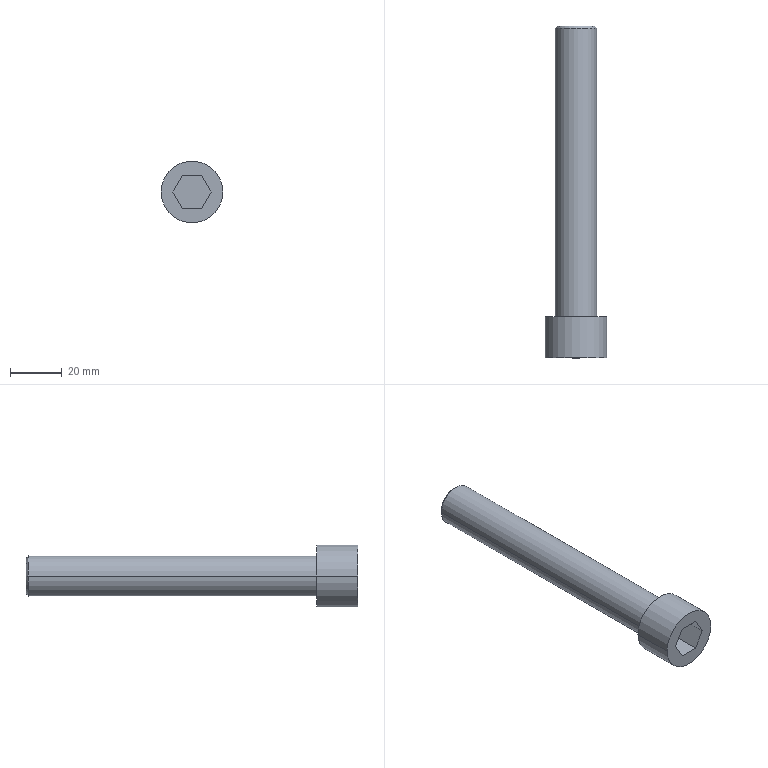Part | STEP file | 4-20.sldasm-Part-98 | 1 solid | 16 faces | box 23.813 x 128.025 x 23.812 mm | volume 27783 mm3 | plane 10 | cylinder 4 | cone 2 | commonest cylinder face diameters 15.875 x2 23.813 x2
STEP:
#1=CARTESIAN_POINT('',(147.,-502.451,200.));
#2=VERTEX_POINT('',#1);
#3=CARTESIAN_POINT('',(133.,-502.451,200.));
#4=VERTEX_POINT('',#3);
#5=CARTESIAN_POINT('',(140.,-502.451,200.));
#6=DIRECTION('',(0.,-1.,0.));
#7=DIRECTION('',(1.,0.,0.));
#8=AXIS2_PLACEMENT_3D('',#5,#6,#7);
#9=CIRCLE('',#8,7.);
#10=EDGE_CURVE('',#2,#4,#9,.T.);
#11=ORIENTED_EDGE('',*,*,#10,.T.);
#12=CARTESIAN_POINT('',(132.063,-503.388,200.));
#13=VERTEX_POINT('',#12);
#14=CARTESIAN_POINT('',(132.063,-503.388,200.));
#15=DIRECTION('',(-0.7071,-0.7071,0.));
#16=VECTOR('',#15,1000.);
#17=LINE('',#14,#16);
#18=EDGE_CURVE('',#4,#13,#17,.T.);
#19=ORIENTED_EDGE('',*,*,#18,.T.);
#20=CARTESIAN_POINT('',(147.938,-503.388,200.));
#21=VERTEX_POINT('',#20);
#22=CARTESIAN_POINT('',(140.,-503.388,200.));
#23=DIRECTION('',(0.,1.,0.));
#24=DIRECTION('',(1.,0.,0.));
#25=AXIS2_PLACEMENT_3D('',#22,#23,#24);
#26=CIRCLE('',#25,7.937);
#27=EDGE_CURVE('',#13,#21,#26,.T.);
#28=ORIENTED_EDGE('',*,*,#27,.T.);
#29=CARTESIAN_POINT('',(147.938,-503.388,200.));
#30=DIRECTION('',(0.7071,-0.7071,0.));
#31=VECTOR('',#30,1000.);
#32=LINE('',#29,#31);
#33=EDGE_CURVE('',#2,#21,#32,.T.);
#34=ORIENTED_EDGE('',*,*,#33,.F.);
#35=EDGE_LOOP('',(#11,#19,#28,#34));
#36=FACE_OUTER_BOUND('',#35,.T.);
#37=CARTESIAN_POINT('',(140.,-503.388,200.));
#38=DIRECTION('',(0.,-1.,0.));
#39=DIRECTION('',(1.,0.,0.));
#40=AXIS2_PLACEMENT_3D('',#37,#38,#39);
#41=CONICAL_SURFACE('',#40,7.937,0.7854);
#42=ADVANCED_FACE('',(#36),#41,.T.);
#43=CARTESIAN_POINT('',(128.094,-614.601,200.));
#44=VERTEX_POINT('',#43);
#45=CARTESIAN_POINT('',(151.906,-614.601,200.));
#46=VERTEX_POINT('',#45);
#47=CARTESIAN_POINT('',(140.,-614.601,200.));
#48=DIRECTION('',(0.,1.,0.));
#49=DIRECTION('',(1.,0.,0.));
#50=AXIS2_PLACEMENT_3D('',#47,#48,#49);
#51=CIRCLE('',#50,11.906);
#52=EDGE_CURVE('',#44,#46,#51,.T.);
#53=ORIENTED_EDGE('',*,*,#52,.F.);
#54=CARTESIAN_POINT('',(128.094,-630.476,200.));
#55=VERTEX_POINT('',#54);
#56=CARTESIAN_POINT('',(128.094,-614.601,200.));
#57=DIRECTION('',(0.,-1.,0.));
#58=VECTOR('',#57,1000.);
#59=LINE('',#56,#58);
#60=EDGE_CURVE('',#44,#55,#59,.T.);
#61=ORIENTED_EDGE('',*,*,#60,.T.);
#62=CARTESIAN_POINT('',(151.906,-630.476,200.));
#63=VERTEX_POINT('',#62);
#64=CARTESIAN_POINT('',(140.,-630.476,200.));
#65=DIRECTION('',(0.,1.,0.));
#66=DIRECTION('',(1.,0.,0.));
#67=AXIS2_PLACEMENT_3D('',#64,#65,#66);
#68=CIRCLE('',#67,11.906);
#69=EDGE_CURVE('',#55,#63,#68,.T.);
#70=ORIENTED_EDGE('',*,*,#69,.T.);
#71=CARTESIAN_POINT('',(151.906,-614.601,200.));
#72=DIRECTION('',(0.,-1.,0.));
#73=VECTOR('',#72,1000.);
#74=LINE('',#71,#73);
#75=EDGE_CURVE('',#46,#63,#74,.T.);
#76=ORIENTED_EDGE('',*,*,#75,.F.);
#77=EDGE_LOOP('',(#53,#61,#70,#76));
#78=FACE_OUTER_BOUND('',#77,.T.);
#79=CARTESIAN_POINT('',(140.,-614.601,200.));
#80=DIRECTION('',(0.,-1.,0.));
#81=DIRECTION('',(1.,0.,0.));
#82=AXIS2_PLACEMENT_3D('',#79,#80,#81);
#83=CYLINDRICAL_SURFACE('',#82,11.906);
#84=ADVANCED_FACE('',(#78),#83,.T.);
#85=CARTESIAN_POINT('',(132.063,-614.601,200.));
#86=VERTEX_POINT('',#85);
#87=CARTESIAN_POINT('',(147.938,-614.601,200.));
#88=VERTEX_POINT('',#87);
#89=CARTESIAN_POINT('',(140.,-614.601,200.));
#90=DIRECTION('',(0.,1.,0.));
#91=DIRECTION('',(1.,0.,0.));
#92=AXIS2_PLACEMENT_3D('',#89,#90,#91);
#93=CIRCLE('',#92,7.937);
#94=EDGE_CURVE('',#86,#88,#93,.T.);
#95=ORIENTED_EDGE('',*,*,#94,.T.);
#96=CARTESIAN_POINT('',(147.938,-614.601,200.));
#97=DIRECTION('',(0.,1.,0.));
#98=VECTOR('',#97,1000.);
#99=LINE('',#96,#98);
#100=EDGE_CURVE('',#88,#21,#99,.T.);
#101=ORIENTED_EDGE('',*,*,#100,.T.);
#102=ORIENTED_EDGE('',*,*,#27,.F.);
#103=CARTESIAN_POINT('',(132.063,-614.601,200.));
#104=DIRECTION('',(0.,1.,0.));
#105=VECTOR('',#104,1000.);
#106=LINE('',#103,#105);
#107=EDGE_CURVE('',#86,#13,#106,.T.);
#108=ORIENTED_EDGE('',*,*,#107,.F.);
#109=EDGE_LOOP('',(#95,#101,#102,#108));
#110=FACE_OUTER_BOUND('',#109,.T.);
#111=CARTESIAN_POINT('',(140.,-614.601,200.));
#112=DIRECTION('',(0.,1.,0.));
#113=DIRECTION('',(-1.,0.,0.));
#114=AXIS2_PLACEMENT_3D('',#111,#112,#113);
#115=CYLINDRICAL_SURFACE('',#114,7.937);
#116=ADVANCED_FACE('',(#110),#115,.T.);
#117=ORIENTED_EDGE('',*,*,#100,.F.);
#118=CARTESIAN_POINT('',(140.,-614.601,200.));
#119=DIRECTION('',(0.,1.,0.));
#120=DIRECTION('',(1.,0.,0.));
#121=AXIS2_PLACEMENT_3D('',#118,#119,#120);
#122=CIRCLE('',#121,7.937);
#123=EDGE_CURVE('',#88,#86,#122,.T.);
#124=ORIENTED_EDGE('',*,*,#123,.T.);
#125=ORIENTED_EDGE('',*,*,#107,.T.);
#126=CARTESIAN_POINT('',(140.,-503.388,200.));
#127=DIRECTION('',(0.,1.,0.));
#128=DIRECTION('',(1.,0.,0.));
#129=AXIS2_PLACEMENT_3D('',#126,#127,#128);
#130=CIRCLE('',#129,7.937);
#131=EDGE_CURVE('',#21,#13,#130,.T.);
#132=ORIENTED_EDGE('',*,*,#131,.F.);
#133=EDGE_LOOP('',(#117,#124,#125,#132));
#134=FACE_OUTER_BOUND('',#133,.T.);
#135=CARTESIAN_POINT('',(140.,-614.601,200.));
#136=DIRECTION('',(0.,1.,0.));
#137=DIRECTION('',(-1.,0.,0.));
#138=AXIS2_PLACEMENT_3D('',#135,#136,#137);
#139=CYLINDRICAL_SURFACE('',#138,7.937);
#140=ADVANCED_FACE('',(#134),#139,.T.);
#141=ORIENTED_EDGE('',*,*,#10,.F.);
#142=CARTESIAN_POINT('',(140.,-502.451,200.));
#143=DIRECTION('',(0.,-1.,0.));
#144=DIRECTION('',(1.,0.,0.));
#145=AXIS2_PLACEMENT_3D('',#142,#143,#144);
#146=CIRCLE('',#145,7.);
#147=EDGE_CURVE('',#4,#2,#146,.T.);
#148=ORIENTED_EDGE('',*,*,#147,.F.);
#149=EDGE_LOOP('',(#141,#148));
#150=FACE_OUTER_BOUND('',#149,.T.);
#151=CARTESIAN_POINT('',(140.,-502.451,200.));
#152=DIRECTION('',(0.,-1.,0.));
#153=DIRECTION('',(1.,0.,0.));
#154=AXIS2_PLACEMENT_3D('',#151,#152,#153);
#155=PLANE('',#154);
#156=ADVANCED_FACE('',(#150),#155,.F.);
#157=CARTESIAN_POINT('',(140.,-614.601,200.));
#158=DIRECTION('',(0.,1.,0.));
#159=DIRECTION('',(1.,0.,0.));
#160=AXIS2_PLACEMENT_3D('',#157,#158,#159);
#161=CIRCLE('',#160,11.906);
#162=EDGE_CURVE('',#46,#44,#161,.T.);
#163=ORIENTED_EDGE('',*,*,#162,.T.);
#164=ORIENTED_EDGE('',*,*,#52,.T.);
#165=EDGE_LOOP('',(#163,#164));
#166=FACE_OUTER_BOUND('',#165,.T.);
#167=ORIENTED_EDGE('',*,*,#94,.F.);
#168=ORIENTED_EDGE('',*,*,#123,.F.);
#169=EDGE_LOOP('',(#167,#168));
#170=FACE_BOUND('',#169,.T.);
#171=CARTESIAN_POINT('',(140.,-614.601,200.));
#172=DIRECTION('',(0.,1.,0.));
#173=DIRECTION('',(-1.,0.,0.));
#174=AXIS2_PLACEMENT_3D('',#171,#172,#173);
#175=PLANE('',#174);
#176=ADVANCED_FACE('',(#166,#170),#175,.T.);
#177=CARTESIAN_POINT('',(136.334,-630.476,206.35));
#178=VERTEX_POINT('',#177);
#179=CARTESIAN_POINT('',(143.666,-630.476,206.35));
#180=VERTEX_POINT('',#179);
#181=CARTESIAN_POINT('',(136.334,-630.476,206.35));
#182=DIRECTION('',(1.,0.,0.));
#183=VECTOR('',#182,1000.);
#184=LINE('',#181,#183);
#185=EDGE_CURVE('',#178,#180,#184,.T.);
#186=ORIENTED_EDGE('',*,*,#185,.T.);
#187=CARTESIAN_POINT('',(147.332,-630.476,200.));
#188=VERTEX_POINT('',#187);
#189=CARTESIAN_POINT('',(143.666,-630.476,206.35));
#190=DIRECTION('',(0.5,0.,-0.866));
#191=VECTOR('',#190,1000.);
#192=LINE('',#189,#191);
#193=EDGE_CURVE('',#180,#188,#192,.T.);
#194=ORIENTED_EDGE('',*,*,#193,.T.);
#195=CARTESIAN_POINT('',(143.666,-630.476,193.65));
#196=VERTEX_POINT('',#195);
#197=CARTESIAN_POINT('',(147.332,-630.476,200.));
#198=DIRECTION('',(-0.5,0.,-0.866));
#199=VECTOR('',#198,1000.);
#200=LINE('',#197,#199);
#201=EDGE_CURVE('',#188,#196,#200,.T.);
#202=ORIENTED_EDGE('',*,*,#201,.T.);
#203=CARTESIAN_POINT('',(136.334,-630.476,193.65));
#204=VERTEX_POINT('',#203);
#205=CARTESIAN_POINT('',(143.666,-630.476,193.65));
#206=DIRECTION('',(-1.,0.,0.));
#207=VECTOR('',#206,1000.);
#208=LINE('',#205,#207);
#209=EDGE_CURVE('',#196,#204,#208,.T.);
#210=ORIENTED_EDGE('',*,*,#209,.T.);
#211=CARTESIAN_POINT('',(132.668,-630.476,200.));
#212=VERTEX_POINT('',#211);
#213=CARTESIAN_POINT('',(136.334,-630.476,193.65));
#214=DIRECTION('',(-0.5,0.,0.866));
#215=VECTOR('',#214,1000.);
#216=LINE('',#213,#215);
#217=EDGE_CURVE('',#204,#212,#216,.T.);
#218=ORIENTED_EDGE('',*,*,#217,.T.);
#219=CARTESIAN_POINT('',(132.668,-630.476,200.));
#220=DIRECTION('',(0.5,0.,0.866));
#221=VECTOR('',#220,1000.);
#222=LINE('',#219,#221);
#223=EDGE_CURVE('',#212,#178,#222,.T.);
#224=ORIENTED_EDGE('',*,*,#223,.T.);
#225=EDGE_LOOP('',(#186,#194,#202,#210,#218,#224));
#226=FACE_BOUND('',#225,.T.);
#227=CARTESIAN_POINT('',(140.,-630.476,200.));
#228=DIRECTION('',(0.,1.,0.));
#229=DIRECTION('',(1.,0.,0.));
#230=AXIS2_PLACEMENT_3D('',#227,#228,#229);
#231=CIRCLE('',#230,11.906);
#232=EDGE_CURVE('',#63,#55,#231,.T.);
#233=ORIENTED_EDGE('',*,*,#232,.F.);
#234=ORIENTED_EDGE('',*,*,#69,.F.);
#235=EDGE_LOOP('',(#233,#234));
#236=FACE_OUTER_BOUND('',#235,.T.);
#237=CARTESIAN_POINT('',(140.,-630.476,200.));
#238=DIRECTION('',(0.,-1.,0.));
#239=DIRECTION('',(1.,0.,0.));
#240=AXIS2_PLACEMENT_3D('',#237,#238,#239);
#241=PLANE('',#240);
#242=ADVANCED_FACE('',(#226,#236),#241,.T.);
#243=ORIENTED_EDGE('',*,*,#60,.F.);
#244=ORIENTED_EDGE('',*,*,#162,.F.);
#245=ORIENTED_EDGE('',*,*,#75,.T.);
#246=ORIENTED_EDGE('',*,*,#232,.T.);
#247=EDGE_LOOP('',(#243,#244,#245,#246));
#248=FACE_OUTER_BOUND('',#247,.T.);
#249=CARTESIAN_POINT('',(140.,-614.601,200.));
#250=DIRECTION('',(0.,-1.,0.));
#251=DIRECTION('',(1.,0.,0.));
#252=AXIS2_PLACEMENT_3D('',#249,#250,#251);
#253=CYLINDRICAL_SURFACE('',#252,11.906);
#254=ADVANCED_FACE('',(#248),#253,.T.);
#255=ORIENTED_EDGE('',*,*,#18,.F.);
#256=ORIENTED_EDGE('',*,*,#147,.T.);
#257=ORIENTED_EDGE('',*,*,#33,.T.);
#258=ORIENTED_EDGE('',*,*,#131,.T.);
#259=EDGE_LOOP('',(#255,#256,#257,#258));
#260=FACE_OUTER_BOUND('',#259,.T.);
#261=CARTESIAN_POINT('',(140.,-503.388,200.));
#262=DIRECTION('',(0.,-1.,0.));
#263=DIRECTION('',(1.,0.,0.));
#264=AXIS2_PLACEMENT_3D('',#261,#262,#263);
#265=CONICAL_SURFACE('',#264,7.937,0.7854);
#266=ADVANCED_FACE('',(#260),#265,.T.);
#267=ORIENTED_EDGE('',*,*,#185,.F.);
#268=CARTESIAN_POINT('',(136.334,-619.999,206.35));
#269=VERTEX_POINT('',#268);
#270=CARTESIAN_POINT('',(136.334,-619.999,206.35));
#271=DIRECTION('',(0.,-1.,0.));
#272=VECTOR('',#271,1000.);
#273=LINE('',#270,#272);
#274=EDGE_CURVE('',#269,#178,#273,.T.);
#275=ORIENTED_EDGE('',*,*,#274,.F.);
#276=CARTESIAN_POINT('',(143.666,-619.999,206.35));
#277=VERTEX_POINT('',#276);
#278=CARTESIAN_POINT('',(136.334,-619.999,206.35));
#279=DIRECTION('',(1.,0.,0.));
#280=VECTOR('',#279,1000.);
#281=LINE('',#278,#280);
#282=EDGE_CURVE('',#269,#277,#281,.T.);
#283=ORIENTED_EDGE('',*,*,#282,.T.);
#284=CARTESIAN_POINT('',(143.666,-619.999,206.35));
#285=DIRECTION('',(0.,-1.,0.));
#286=VECTOR('',#285,1000.);
#287=LINE('',#284,#286);
#288=EDGE_CURVE('',#277,#180,#287,.T.);
#289=ORIENTED_EDGE('',*,*,#288,.T.);
#290=EDGE_LOOP('',(#267,#275,#283,#289));
#291=FACE_OUTER_BOUND('',#290,.T.);
#292=CARTESIAN_POINT('',(136.334,-619.999,206.35));
#293=DIRECTION('',(0.,0.,1.));
#294=DIRECTION('',(0.,1.,0.));
#295=AXIS2_PLACEMENT_3D('',#292,#293,#294);
#296=PLANE('',#295);
#297=ADVANCED_FACE('',(#291),#296,.F.);
#298=ORIENTED_EDGE('',*,*,#193,.F.);
#299=ORIENTED_EDGE('',*,*,#288,.F.);
#300=CARTESIAN_POINT('',(147.332,-619.999,200.));
#301=VERTEX_POINT('',#300);
#302=CARTESIAN_POINT('',(143.666,-619.999,206.35));
#303=DIRECTION('',(0.5,0.,-0.866));
#304=VECTOR('',#303,1000.);
#305=LINE('',#302,#304);
#306=EDGE_CURVE('',#277,#301,#305,.T.);
#307=ORIENTED_EDGE('',*,*,#306,.T.);
#308=CARTESIAN_POINT('',(147.332,-619.999,200.));
#309=DIRECTION('',(0.,-1.,0.));
#310=VECTOR('',#309,1000.);
#311=LINE('',#308,#310);
#312=EDGE_CURVE('',#301,#188,#311,.T.);
#313=ORIENTED_EDGE('',*,*,#312,.T.);
#314=EDGE_LOOP('',(#298,#299,#307,#313));
#315=FACE_OUTER_BOUND('',#314,.T.);
#316=CARTESIAN_POINT('',(143.666,-619.999,206.35));
#317=DIRECTION('',(0.866,0.,0.5));
#318=DIRECTION('',(0.5,0.,-0.866));
#319=AXIS2_PLACEMENT_3D('',#316,#317,#318);
#320=PLANE('',#319);
#321=ADVANCED_FACE('',(#315),#320,.F.);
#322=ORIENTED_EDGE('',*,*,#201,.F.);
#323=ORIENTED_EDGE('',*,*,#312,.F.);
#324=CARTESIAN_POINT('',(143.666,-619.999,193.65));
#325=VERTEX_POINT('',#324);
#326=CARTESIAN_POINT('',(147.332,-619.999,200.));
#327=DIRECTION('',(-0.5,0.,-0.866));
#328=VECTOR('',#327,1000.);
#329=LINE('',#326,#328);
#330=EDGE_CURVE('',#301,#325,#329,.T.);
#331=ORIENTED_EDGE('',*,*,#330,.T.);
#332=CARTESIAN_POINT('',(143.666,-619.999,193.65));
#333=DIRECTION('',(0.,-1.,0.));
#334=VECTOR('',#333,1000.);
#335=LINE('',#332,#334);
#336=EDGE_CURVE('',#325,#196,#335,.T.);
#337=ORIENTED_EDGE('',*,*,#336,.T.);
#338=EDGE_LOOP('',(#322,#323,#331,#337));
#339=FACE_OUTER_BOUND('',#338,.T.);
#340=CARTESIAN_POINT('',(147.332,-619.999,200.));
#341=DIRECTION('',(0.866,0.,-0.5));
#342=DIRECTION('',(-0.5,0.,-0.866));
#343=AXIS2_PLACEMENT_3D('',#340,#341,#342);
#344=PLANE('',#343);
#345=ADVANCED_FACE('',(#339),#344,.F.);
#346=ORIENTED_EDGE('',*,*,#209,.F.);
#347=ORIENTED_EDGE('',*,*,#336,.F.);
#348=CARTESIAN_POINT('',(136.334,-619.999,193.65));
#349=VERTEX_POINT('',#348);
#350=CARTESIAN_POINT('',(143.666,-619.999,193.65));
#351=DIRECTION('',(-1.,0.,0.));
#352=VECTOR('',#351,1000.);
#353=LINE('',#350,#352);
#354=EDGE_CURVE('',#325,#349,#353,.T.);
#355=ORIENTED_EDGE('',*,*,#354,.T.);
#356=CARTESIAN_POINT('',(136.334,-619.999,193.65));
#357=DIRECTION('',(0.,-1.,0.));
#358=VECTOR('',#357,1000.);
#359=LINE('',#356,#358);
#360=EDGE_CURVE('',#349,#204,#359,.T.);
#361=ORIENTED_EDGE('',*,*,#360,.T.);
#362=EDGE_LOOP('',(#346,#347,#355,#361));
#363=FACE_OUTER_BOUND('',#362,.T.);
#364=CARTESIAN_POINT('',(143.666,-619.999,193.65));
#365=DIRECTION('',(0.,0.,-1.));
#366=DIRECTION('',(0.,-1.,0.));
#367=AXIS2_PLACEMENT_3D('',#364,#365,#366);
#368=PLANE('',#367);
#369=ADVANCED_FACE('',(#363),#368,.F.);
#370=ORIENTED_EDGE('',*,*,#217,.F.);
#371=ORIENTED_EDGE('',*,*,#360,.F.);
#372=CARTESIAN_POINT('',(132.668,-619.999,200.));
#373=VERTEX_POINT('',#372);
#374=CARTESIAN_POINT('',(136.334,-619.999,193.65));
#375=DIRECTION('',(-0.5,0.,0.866));
#376=VECTOR('',#375,1000.);
#377=LINE('',#374,#376);
#378=EDGE_CURVE('',#349,#373,#377,.T.);
#379=ORIENTED_EDGE('',*,*,#378,.T.);
#380=CARTESIAN_POINT('',(132.668,-619.999,200.));
#381=DIRECTION('',(0.,-1.,0.));
#382=VECTOR('',#381,1000.);
#383=LINE('',#380,#382);
#384=EDGE_CURVE('',#373,#212,#383,.T.);
#385=ORIENTED_EDGE('',*,*,#384,.T.);
#386=EDGE_LOOP('',(#370,#371,#379,#385));
#387=FACE_OUTER_BOUND('',#386,.T.);
#388=CARTESIAN_POINT('',(136.334,-619.999,193.65));
#389=DIRECTION('',(-0.866,0.,-0.5));
#390=DIRECTION('',(-0.5,0.,0.866));
#391=AXIS2_PLACEMENT_3D('',#388,#389,#390);
#392=PLANE('',#391);
#393=ADVANCED_FACE('',(#387),#392,.F.);
#394=ORIENTED_EDGE('',*,*,#223,.F.);
#395=ORIENTED_EDGE('',*,*,#384,.F.);
#396=CARTESIAN_POINT('',(132.668,-619.999,200.));
#397=DIRECTION('',(0.5,0.,0.866));
#398=VECTOR('',#397,1000.);
#399=LINE('',#396,#398);
#400=EDGE_CURVE('',#373,#269,#399,.T.);
#401=ORIENTED_EDGE('',*,*,#400,.T.);
#402=ORIENTED_EDGE('',*,*,#274,.T.);
#403=EDGE_LOOP('',(#394,#395,#401,#402));
#404=FACE_OUTER_BOUND('',#403,.T.);
#405=CARTESIAN_POINT('',(132.668,-619.999,200.));
#406=DIRECTION('',(-0.866,0.,0.5));
#407=DIRECTION('',(0.5,0.,0.866));
#408=AXIS2_PLACEMENT_3D('',#405,#406,#407);
#409=PLANE('',#408);
#410=ADVANCED_FACE('',(#404),#409,.F.);
#411=ORIENTED_EDGE('',*,*,#282,.F.);
#412=ORIENTED_EDGE('',*,*,#400,.F.);
#413=ORIENTED_EDGE('',*,*,#378,.F.);
#414=ORIENTED_EDGE('',*,*,#354,.F.);
#415=ORIENTED_EDGE('',*,*,#330,.F.);
#416=ORIENTED_EDGE('',*,*,#306,.F.);
#417=EDGE_LOOP('',(#411,#412,#413,#414,#415,#416));
#418=FACE_OUTER_BOUND('',#417,.T.);
#419=CARTESIAN_POINT('',(143.666,-619.999,206.35));
#420=DIRECTION('',(0.,-1.,0.));
#421=DIRECTION('',(1.,0.,0.));
#422=AXIS2_PLACEMENT_3D('',#419,#420,#421);
#423=PLANE('',#422);
#424=ADVANCED_FACE('',(#418),#423,.T.);
#425=CLOSED_SHELL('',(#42,#84,#116,#140,#156,#176,#242,#254,#266,#297,#321,#345,#369,#393,#410,#424));
#426=MANIFOLD_SOLID_BREP('',#425);
#427=CARTESIAN_POINT('',(0.,0.,0.));
#428=DIRECTION('',(0.,0.,1.));
#429=DIRECTION('',(1.,0.,0.));
#430=AXIS2_PLACEMENT_3D('',#427,#428,#429);
#431=(LENGTH_UNIT()NAMED_UNIT(*)SI_UNIT(.MILLI.,.METRE.));
#432=UNCERTAINTY_MEASURE_WITH_UNIT(LENGTH_MEASURE(0.00001),#431,'','');
#433=(NAMED_UNIT(*)PLANE_ANGLE_UNIT()SI_UNIT($,.RADIAN.));
#434=(NAMED_UNIT(*)SI_UNIT($,.STERADIAN.)SOLID_ANGLE_UNIT());
#435=(GEOMETRIC_REPRESENTATION_CONTEXT(3)GLOBAL_UNCERTAINTY_ASSIGNED_CONTEXT((#432))GLOBAL_UNIT_ASSIGNED_CONTEXT((#431,#433,#434))REPRESENTATION_CONTEXT('',''));
#436=ADVANCED_BREP_SHAPE_REPRESENTATION('',(#426,#430),#435);